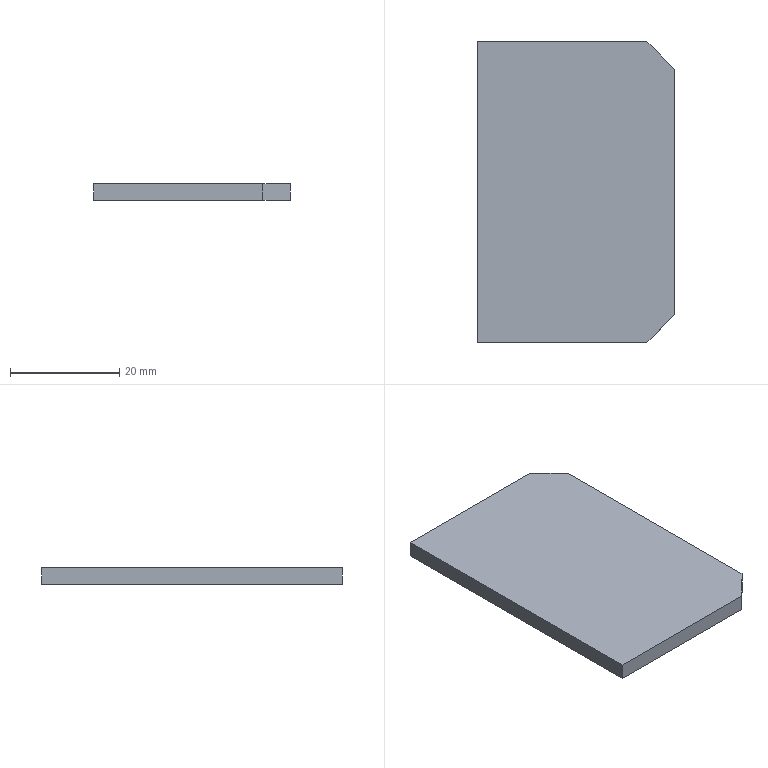Part | SolidWorks | features Chamfer 1, Extrusion 1 | 1 solid | 8 faces | box 36 x 55 x 3 mm | volume 5865 mm3 | plane 8
STEP:
#1=CARTESIAN_POINT('',(0.,55.,0.));
#2=VERTEX_POINT('',#1);
#3=CARTESIAN_POINT('',(0.,0.,0.));
#4=VERTEX_POINT('',#3);
#5=CARTESIAN_POINT('',(0.,55.,0.));
#6=DIRECTION('',(0.,-1.,0.));
#7=VECTOR('',#6,1000.);
#8=LINE('',#5,#7);
#9=EDGE_CURVE('',#2,#4,#8,.T.);
#10=ORIENTED_EDGE('',*,*,#9,.T.);
#11=CARTESIAN_POINT('',(0.,0.,3.));
#12=VERTEX_POINT('',#11);
#13=CARTESIAN_POINT('',(0.,0.,3.));
#14=DIRECTION('',(0.,0.,-1.));
#15=VECTOR('',#14,1000.);
#16=LINE('',#13,#15);
#17=EDGE_CURVE('',#12,#4,#16,.T.);
#18=ORIENTED_EDGE('',*,*,#17,.F.);
#19=CARTESIAN_POINT('',(0.,55.,3.));
#20=VERTEX_POINT('',#19);
#21=CARTESIAN_POINT('',(0.,55.,3.));
#22=DIRECTION('',(0.,-1.,0.));
#23=VECTOR('',#22,1000.);
#24=LINE('',#21,#23);
#25=EDGE_CURVE('',#20,#12,#24,.T.);
#26=ORIENTED_EDGE('',*,*,#25,.F.);
#27=CARTESIAN_POINT('',(0.,55.,3.));
#28=DIRECTION('',(0.,0.,-1.));
#29=VECTOR('',#28,1000.);
#30=LINE('',#27,#29);
#31=EDGE_CURVE('',#20,#2,#30,.T.);
#32=ORIENTED_EDGE('',*,*,#31,.T.);
#33=EDGE_LOOP('',(#10,#18,#26,#32));
#34=FACE_OUTER_BOUND('',#33,.T.);
#35=CARTESIAN_POINT('',(0.,55.,3.));
#36=DIRECTION('',(1.,0.,0.));
#37=DIRECTION('',(0.,1.,0.));
#38=AXIS2_PLACEMENT_3D('',#35,#36,#37);
#39=PLANE('',#38);
#40=ADVANCED_FACE('',(#34),#39,.F.);
#41=CARTESIAN_POINT('',(31.,0.,0.));
#42=VERTEX_POINT('',#41);
#43=CARTESIAN_POINT('',(0.,0.,0.));
#44=DIRECTION('',(1.,0.,0.));
#45=VECTOR('',#44,1000.);
#46=LINE('',#43,#45);
#47=EDGE_CURVE('',#4,#42,#46,.T.);
#48=ORIENTED_EDGE('',*,*,#47,.T.);
#49=CARTESIAN_POINT('',(31.,0.,3.));
#50=VERTEX_POINT('',#49);
#51=CARTESIAN_POINT('',(31.,0.,3.));
#52=DIRECTION('',(0.,0.,1.));
#53=VECTOR('',#52,1000.);
#54=LINE('',#51,#53);
#55=EDGE_CURVE('',#42,#50,#54,.T.);
#56=ORIENTED_EDGE('',*,*,#55,.T.);
#57=CARTESIAN_POINT('',(0.,0.,3.));
#58=DIRECTION('',(1.,0.,0.));
#59=VECTOR('',#58,1000.);
#60=LINE('',#57,#59);
#61=EDGE_CURVE('',#12,#50,#60,.T.);
#62=ORIENTED_EDGE('',*,*,#61,.F.);
#63=ORIENTED_EDGE('',*,*,#17,.T.);
#64=EDGE_LOOP('',(#48,#56,#62,#63));
#65=FACE_OUTER_BOUND('',#64,.T.);
#66=CARTESIAN_POINT('',(0.,0.,3.));
#67=DIRECTION('',(0.,1.,0.));
#68=DIRECTION('',(0.,0.,1.));
#69=AXIS2_PLACEMENT_3D('',#66,#67,#68);
#70=PLANE('',#69);
#71=ADVANCED_FACE('',(#65),#70,.F.);
#72=CARTESIAN_POINT('',(36.,5.,3.));
#73=VERTEX_POINT('',#72);
#74=CARTESIAN_POINT('',(36.,50.,3.));
#75=VERTEX_POINT('',#74);
#76=CARTESIAN_POINT('',(36.,0.,3.));
#77=DIRECTION('',(0.,1.,0.));
#78=VECTOR('',#77,1000.);
#79=LINE('',#76,#78);
#80=EDGE_CURVE('',#73,#75,#79,.T.);
#81=ORIENTED_EDGE('',*,*,#80,.F.);
#82=CARTESIAN_POINT('',(36.,5.,0.));
#83=VERTEX_POINT('',#82);
#84=CARTESIAN_POINT('',(36.,5.,3.));
#85=DIRECTION('',(0.,0.,-1.));
#86=VECTOR('',#85,1000.);
#87=LINE('',#84,#86);
#88=EDGE_CURVE('',#73,#83,#87,.T.);
#89=ORIENTED_EDGE('',*,*,#88,.T.);
#90=CARTESIAN_POINT('',(36.,50.,0.));
#91=VERTEX_POINT('',#90);
#92=CARTESIAN_POINT('',(36.,0.,0.));
#93=DIRECTION('',(0.,1.,0.));
#94=VECTOR('',#93,1000.);
#95=LINE('',#92,#94);
#96=EDGE_CURVE('',#83,#91,#95,.T.);
#97=ORIENTED_EDGE('',*,*,#96,.T.);
#98=CARTESIAN_POINT('',(36.,50.,3.));
#99=DIRECTION('',(0.,0.,1.));
#100=VECTOR('',#99,1000.);
#101=LINE('',#98,#100);
#102=EDGE_CURVE('',#91,#75,#101,.T.);
#103=ORIENTED_EDGE('',*,*,#102,.T.);
#104=EDGE_LOOP('',(#81,#89,#97,#103));
#105=FACE_OUTER_BOUND('',#104,.T.);
#106=CARTESIAN_POINT('',(36.,0.,3.));
#107=DIRECTION('',(-1.,0.,0.));
#108=DIRECTION('',(0.,0.,1.));
#109=AXIS2_PLACEMENT_3D('',#106,#107,#108);
#110=PLANE('',#109);
#111=ADVANCED_FACE('',(#105),#110,.F.);
#112=CARTESIAN_POINT('',(31.,55.,3.));
#113=VERTEX_POINT('',#112);
#114=CARTESIAN_POINT('',(36.,55.,3.));
#115=DIRECTION('',(-1.,0.,0.));
#116=VECTOR('',#115,1000.);
#117=LINE('',#114,#116);
#118=EDGE_CURVE('',#113,#20,#117,.T.);
#119=ORIENTED_EDGE('',*,*,#118,.F.);
#120=CARTESIAN_POINT('',(31.,55.,0.));
#121=VERTEX_POINT('',#120);
#122=CARTESIAN_POINT('',(31.,55.,3.));
#123=DIRECTION('',(0.,0.,-1.));
#124=VECTOR('',#123,1000.);
#125=LINE('',#122,#124);
#126=EDGE_CURVE('',#113,#121,#125,.T.);
#127=ORIENTED_EDGE('',*,*,#126,.T.);
#128=CARTESIAN_POINT('',(36.,55.,0.));
#129=DIRECTION('',(-1.,0.,0.));
#130=VECTOR('',#129,1000.);
#131=LINE('',#128,#130);
#132=EDGE_CURVE('',#121,#2,#131,.T.);
#133=ORIENTED_EDGE('',*,*,#132,.T.);
#134=ORIENTED_EDGE('',*,*,#31,.F.);
#135=EDGE_LOOP('',(#119,#127,#133,#134));
#136=FACE_OUTER_BOUND('',#135,.T.);
#137=CARTESIAN_POINT('',(36.,55.,3.));
#138=DIRECTION('',(0.,-1.,0.));
#139=DIRECTION('',(1.,0.,0.));
#140=AXIS2_PLACEMENT_3D('',#137,#138,#139);
#141=PLANE('',#140);
#142=ADVANCED_FACE('',(#136),#141,.F.);
#143=ORIENTED_EDGE('',*,*,#61,.T.);
#144=CARTESIAN_POINT('',(15.5,-15.5,3.));
#145=DIRECTION('',(0.7071,0.7071,0.));
#146=VECTOR('',#145,1000.);
#147=LINE('',#144,#146);
#148=EDGE_CURVE('',#50,#73,#147,.T.);
#149=ORIENTED_EDGE('',*,*,#148,.T.);
#150=ORIENTED_EDGE('',*,*,#80,.T.);
#151=CARTESIAN_POINT('',(43.,43.,3.));
#152=DIRECTION('',(-0.7071,0.7071,0.));
#153=VECTOR('',#152,1000.);
#154=LINE('',#151,#153);
#155=EDGE_CURVE('',#75,#113,#154,.T.);
#156=ORIENTED_EDGE('',*,*,#155,.T.);
#157=ORIENTED_EDGE('',*,*,#118,.T.);
#158=ORIENTED_EDGE('',*,*,#25,.T.);
#159=EDGE_LOOP('',(#143,#149,#150,#156,#157,#158));
#160=FACE_OUTER_BOUND('',#159,.T.);
#161=CARTESIAN_POINT('',(0.,0.,3.));
#162=DIRECTION('',(0.,0.,1.));
#163=DIRECTION('',(1.,0.,0.));
#164=AXIS2_PLACEMENT_3D('',#161,#162,#163);
#165=PLANE('',#164);
#166=ADVANCED_FACE('',(#160),#165,.T.);
#167=ORIENTED_EDGE('',*,*,#96,.F.);
#168=CARTESIAN_POINT('',(36.,5.,0.));
#169=DIRECTION('',(-0.7071,-0.7071,0.));
#170=VECTOR('',#169,1000.);
#171=LINE('',#168,#170);
#172=EDGE_CURVE('',#83,#42,#171,.T.);
#173=ORIENTED_EDGE('',*,*,#172,.T.);
#174=ORIENTED_EDGE('',*,*,#47,.F.);
#175=ORIENTED_EDGE('',*,*,#9,.F.);
#176=ORIENTED_EDGE('',*,*,#132,.F.);
#177=CARTESIAN_POINT('',(31.,55.,0.));
#178=DIRECTION('',(0.7071,-0.7071,0.));
#179=VECTOR('',#178,1000.);
#180=LINE('',#177,#179);
#181=EDGE_CURVE('',#121,#91,#180,.T.);
#182=ORIENTED_EDGE('',*,*,#181,.T.);
#183=EDGE_LOOP('',(#167,#173,#174,#175,#176,#182));
#184=FACE_OUTER_BOUND('',#183,.T.);
#185=CARTESIAN_POINT('',(0.,0.,0.));
#186=DIRECTION('',(0.,0.,1.));
#187=DIRECTION('',(1.,0.,0.));
#188=AXIS2_PLACEMENT_3D('',#185,#186,#187);
#189=PLANE('',#188);
#190=ADVANCED_FACE('',(#184),#189,.F.);
#191=ORIENTED_EDGE('',*,*,#148,.F.);
#192=ORIENTED_EDGE('',*,*,#55,.F.);
#193=ORIENTED_EDGE('',*,*,#172,.F.);
#194=ORIENTED_EDGE('',*,*,#88,.F.);
#195=EDGE_LOOP('',(#191,#192,#193,#194));
#196=FACE_OUTER_BOUND('',#195,.T.);
#197=CARTESIAN_POINT('',(36.,5.,3.));
#198=DIRECTION('',(-0.7071,0.7071,0.));
#199=DIRECTION('',(0.,0.,-1.));
#200=AXIS2_PLACEMENT_3D('',#197,#198,#199);
#201=PLANE('',#200);
#202=ADVANCED_FACE('',(#196),#201,.F.);
#203=ORIENTED_EDGE('',*,*,#155,.F.);
#204=ORIENTED_EDGE('',*,*,#102,.F.);
#205=ORIENTED_EDGE('',*,*,#181,.F.);
#206=ORIENTED_EDGE('',*,*,#126,.F.);
#207=EDGE_LOOP('',(#203,#204,#205,#206));
#208=FACE_OUTER_BOUND('',#207,.T.);
#209=CARTESIAN_POINT('',(31.,55.,3.));
#210=DIRECTION('',(-0.7071,-0.7071,0.));
#211=DIRECTION('',(0.,0.,-1.));
#212=AXIS2_PLACEMENT_3D('',#209,#210,#211);
#213=PLANE('',#212);
#214=ADVANCED_FACE('',(#208),#213,.F.);
#215=CLOSED_SHELL('',(#40,#71,#111,#142,#166,#190,#202,#214));
#216=MANIFOLD_SOLID_BREP('',#215);
#217=CARTESIAN_POINT('',(0.,0.,0.));
#218=DIRECTION('',(0.,0.,1.));
#219=DIRECTION('',(1.,0.,0.));
#220=AXIS2_PLACEMENT_3D('',#217,#218,#219);
#221=(LENGTH_UNIT()NAMED_UNIT(*)SI_UNIT(.MILLI.,.METRE.));
#222=UNCERTAINTY_MEASURE_WITH_UNIT(LENGTH_MEASURE(0.00001),#221,'','');
#223=(NAMED_UNIT(*)PLANE_ANGLE_UNIT()SI_UNIT($,.RADIAN.));
#224=(NAMED_UNIT(*)SI_UNIT($,.STERADIAN.)SOLID_ANGLE_UNIT());
#225=(GEOMETRIC_REPRESENTATION_CONTEXT(3)GLOBAL_UNCERTAINTY_ASSIGNED_CONTEXT((#222))GLOBAL_UNIT_ASSIGNED_CONTEXT((#221,#223,#224))REPRESENTATION_CONTEXT('',''));
#226=ADVANCED_BREP_SHAPE_REPRESENTATION('',(#216,#220),#225);